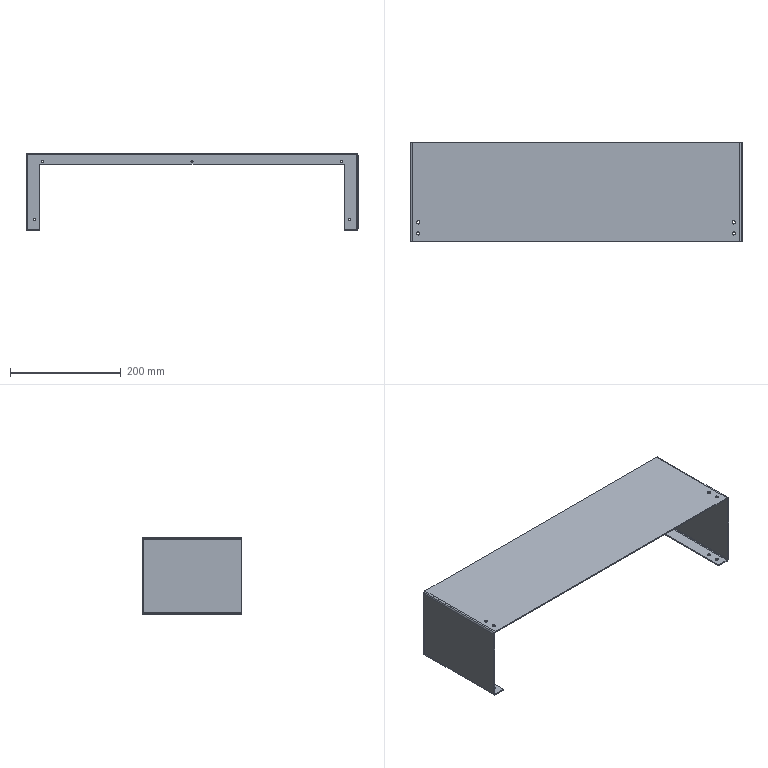Part | STEP file | CHAIN.COVER.1.stp | 1 solid | 58 faces | box 600 x 180 x 140 mm | volume 361793 mm3 | cylinder 32 | spline 18 | plane 8 | commonest cylinder face diameters 4 x16 6 x8 8 x8